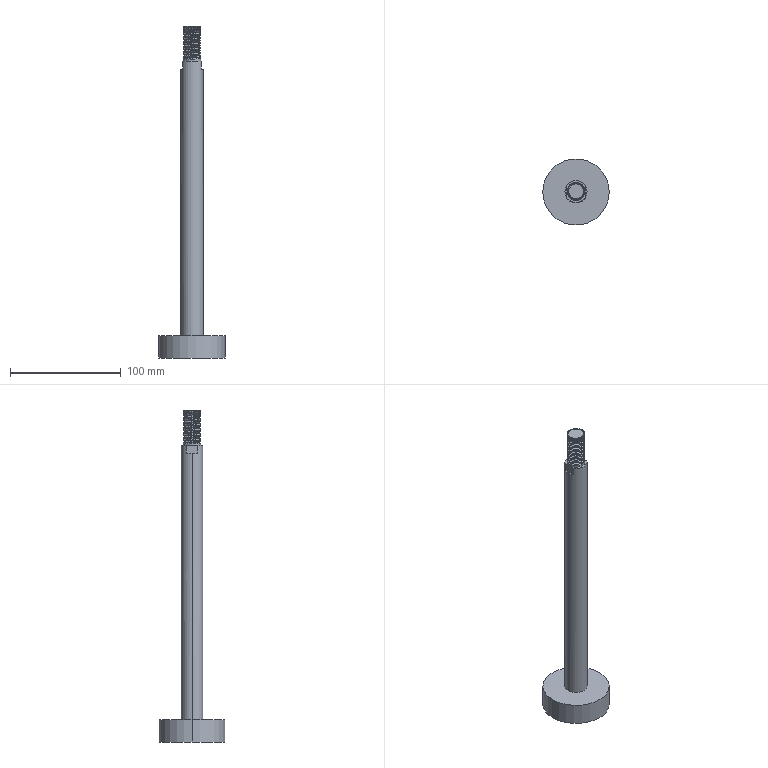Part | NX | 3 solids | 59 faces | box 60 x 60 x 300 mm | volume 139937 mm3 | cylinder 45 | plane 12 | spline 2 | commonest cylinder face diameters 16 x41 20 x2 60 x2